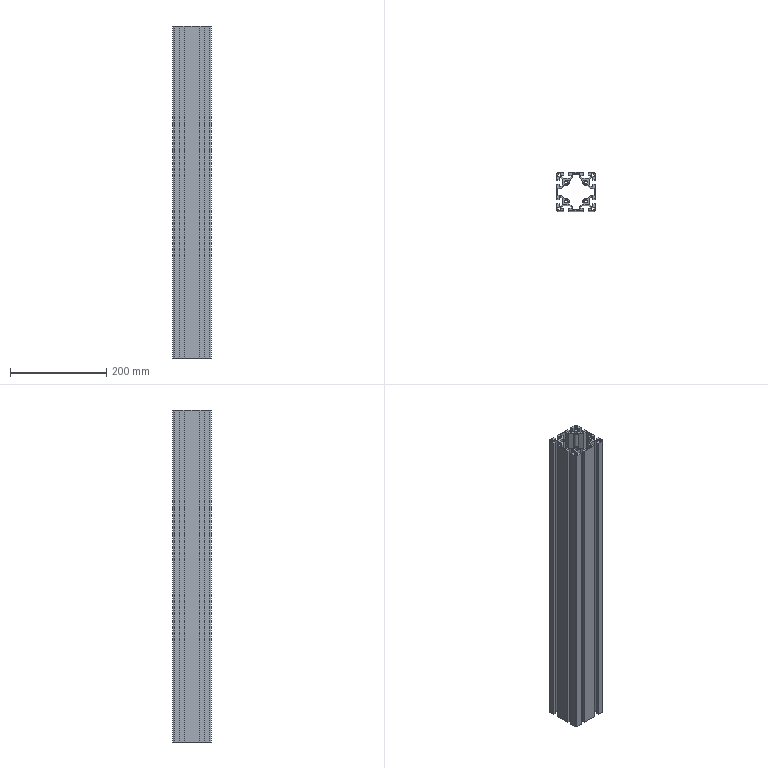Part | NX | 1 solid | 156 faces | box 80 x 80 x 690 mm | volume 1208882 mm3 | plane 122 | cylinder 34 | commonest cylinder face diameters 2 x16 6.8 x8 11.8 x6 5.64 x4